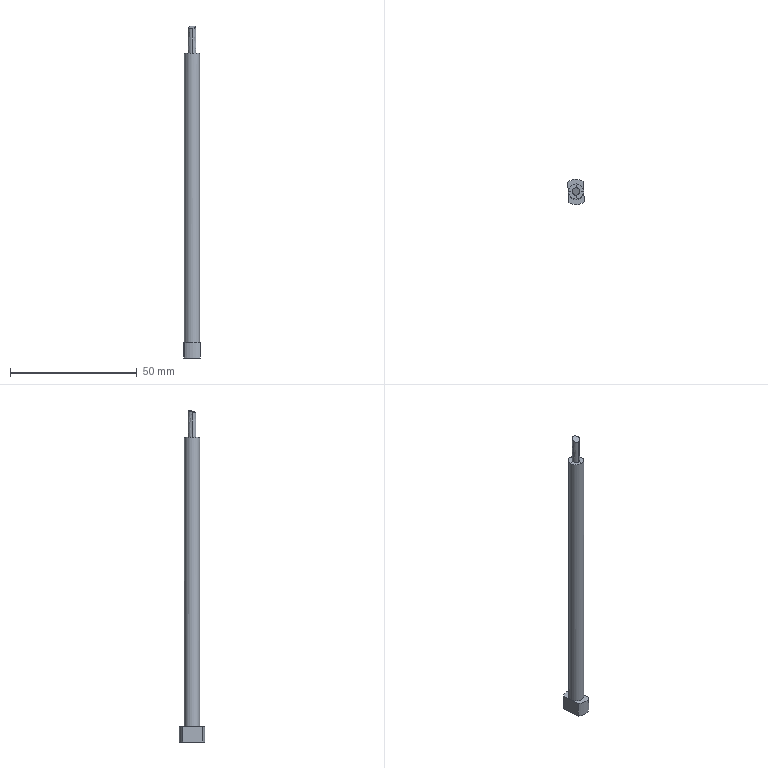Part | STEP file | 车灯-后视镜_id590_x_t | 1 solid | 16 faces | box 6.638 x 10 x 131.059 mm | volume 3645 mm3 | plane 8 | spline 5 | cylinder 3 | commonest cylinder face diameters 10 x2 6 x1
STEP:
#1=CARTESIAN_POINT('',(14.563,-72.692,45.992));
#2=VERTEX_POINT('',#1);
#3=CARTESIAN_POINT('',(11.568,-69.68,45.99));
#4=VERTEX_POINT('',#3);
#5=CARTESIAN_POINT('',(11.563,-72.687,45.992));
#6=DIRECTION('',(-0.00001772,-0.00006118,1.));
#7=DIRECTION('',(0.2782,0.9605,0.00006369));
#8=AXIS2_PLACEMENT_3D('',#5,#6,#7);
#9=ELLIPSE('',#8,3.,3.);
#10=EDGE_CURVE('',#2,#4,#9,.T.);
#11=ORIENTED_EDGE('',*,*,#10,.F.);
#12=CARTESIAN_POINT('',(11.575,-75.7,45.991));
#13=VERTEX_POINT('',#12);
#14=CARTESIAN_POINT('',(11.563,-72.687,45.992));
#15=DIRECTION('',(-0.00004877,0.00005142,-1.));
#16=DIRECTION('',(-0.6881,0.7256,0.00007087));
#17=AXIS2_PLACEMENT_3D('',#14,#15,#16);
#18=ELLIPSE('',#17,3.,3.);
#19=EDGE_CURVE('',#2,#13,#18,.T.);
#20=ORIENTED_EDGE('',*,*,#19,.T.);
#21=CARTESIAN_POINT('',(8.555,-72.692,45.989));
#22=VERTEX_POINT('',#21);
#23=CARTESIAN_POINT('',(8.555,-72.692,45.992));
#24=CARTESIAN_POINT('',(8.556,-73.526,45.992));
#25=CARTESIAN_POINT('',(8.85,-74.236,45.992));
#26=CARTESIAN_POINT('',(10.027,-75.412,45.992));
#27=CARTESIAN_POINT('',(10.738,-75.707,45.992));
#28=CARTESIAN_POINT('',(11.57,-75.707,45.992));
#29=B_SPLINE_CURVE_WITH_KNOTS('',3,(#23,#24,#25,#26,#27,#28),.UNSPECIFIED.,.F.,.F.,(4,2,4),(0.,0.5,1.),.UNSPECIFIED.);
#30=EDGE_CURVE('',#22,#13,#29,.T.);
#31=ORIENTED_EDGE('',*,*,#30,.F.);
#32=CARTESIAN_POINT('',(8.563,-72.692,45.992));
#33=CARTESIAN_POINT('',(8.562,-71.905,45.992));
#34=CARTESIAN_POINT('',(8.885,-71.122,45.992));
#35=CARTESIAN_POINT('',(9.998,-70.01,45.992));
#36=CARTESIAN_POINT('',(10.781,-69.686,45.992));
#37=CARTESIAN_POINT('',(11.568,-69.687,45.992));
#38=B_SPLINE_CURVE_WITH_KNOTS('',3,(#32,#33,#34,#35,#36,#37),.UNSPECIFIED.,.F.,.F.,(4,2,4),(0.,0.5,1.),.UNSPECIFIED.);
#39=EDGE_CURVE('',#22,#4,#38,.T.);
#40=ORIENTED_EDGE('',*,*,#39,.T.);
#41=EDGE_LOOP('',(#11,#20,#31,#40));
#42=FACE_BOUND('',#41,.T.);
#43=CARTESIAN_POINT('',(14.563,-72.687,-68.25));
#44=VERTEX_POINT('',#43);
#45=CARTESIAN_POINT('',(11.563,-72.687,-68.25));
#46=DIRECTION('',(0.,0.,-1.));
#47=DIRECTION('',(1.,0.,0.));
#48=AXIS2_PLACEMENT_3D('',#45,#46,#47);
#49=CIRCLE('',#48,3.);
#50=EDGE_CURVE('',#44,#44,#49,.T.);
#51=ORIENTED_EDGE('',*,*,#50,.F.);
#52=EDGE_LOOP('',(#51));
#53=FACE_BOUND('',#52,.T.);
#54=CARTESIAN_POINT('',(11.563,-72.687,45.992));
#55=DIRECTION('',(0.,0.,1.));
#56=DIRECTION('',(1.,0.,0.));
#57=AXIS2_PLACEMENT_3D('',#54,#55,#56);
#58=CYLINDRICAL_SURFACE('',#57,3.);
#59=ADVANCED_FACE('',(#42,#53),#58,.T.);
#60=CARTESIAN_POINT('',(11.567,-71.184,56.788));
#61=VERTEX_POINT('',#60);
#62=CARTESIAN_POINT('',(11.275,-71.215,56.744));
#63=VERTEX_POINT('',#62);
#64=CARTESIAN_POINT('',(11.567,-71.184,56.788));
#65=CARTESIAN_POINT('',(11.469,-71.195,56.774));
#66=CARTESIAN_POINT('',(11.372,-71.205,56.761));
#67=CARTESIAN_POINT('',(11.275,-71.216,56.747));
#68=B_SPLINE_CURVE_WITH_KNOTS('',3,(#64,#65,#66,#67),.UNSPECIFIED.,.F.,.F.,(4,4),(0.,1.),.UNSPECIFIED.);
#69=EDGE_CURVE('',#61,#63,#68,.T.);
#70=ORIENTED_EDGE('',*,*,#69,.T.);
#71=CARTESIAN_POINT('',(10.857,-71.372,56.641));
#72=VERTEX_POINT('',#71);
#73=CARTESIAN_POINT('',(11.275,-71.216,56.747));
#74=CARTESIAN_POINT('',(11.135,-71.269,56.714));
#75=CARTESIAN_POINT('',(10.995,-71.322,56.681));
#76=CARTESIAN_POINT('',(10.856,-71.374,56.648));
#77=B_SPLINE_CURVE_WITH_KNOTS('',3,(#73,#74,#75,#76),.UNSPECIFIED.,.F.,.F.,(4,4),(0.,1.),.UNSPECIFIED.);
#78=EDGE_CURVE('',#63,#72,#77,.T.);
#79=ORIENTED_EDGE('',*,*,#78,.T.);
#80=CARTESIAN_POINT('',(10.059,-72.692,56.102));
#81=VERTEX_POINT('',#80);
#82=CARTESIAN_POINT('',(10.856,-71.374,56.648));
#83=CARTESIAN_POINT('',(10.323,-71.672,56.488));
#84=CARTESIAN_POINT('',(10.059,-72.113,56.305));
#85=CARTESIAN_POINT('',(10.059,-72.692,56.102));
#86=B_SPLINE_CURVE_WITH_KNOTS('',3,(#82,#83,#84,#85),.UNSPECIFIED.,.F.,.F.,(4,4),(0.,1.),.UNSPECIFIED.);
#87=EDGE_CURVE('',#72,#81,#86,.T.);
#88=ORIENTED_EDGE('',*,*,#87,.T.);
#89=CARTESIAN_POINT('',(10.061,-72.772,56.074));
#90=VERTEX_POINT('',#89);
#91=CARTESIAN_POINT('',(10.059,-72.692,56.102));
#92=CARTESIAN_POINT('',(10.06,-72.719,56.093));
#93=CARTESIAN_POINT('',(10.061,-72.746,56.084));
#94=CARTESIAN_POINT('',(10.061,-72.772,56.074));
#95=B_SPLINE_CURVE_WITH_KNOTS('',3,(#91,#92,#93,#94),.UNSPECIFIED.,.F.,.F.,(4,4),(0.,1.),.UNSPECIFIED.);
#96=EDGE_CURVE('',#81,#90,#95,.T.);
#97=ORIENTED_EDGE('',*,*,#96,.T.);
#98=CARTESIAN_POINT('',(11.099,-74.121,55.708));
#99=VERTEX_POINT('',#98);
#100=CARTESIAN_POINT('',(10.061,-72.772,56.074));
#101=CARTESIAN_POINT('',(10.081,-73.101,55.961));
#102=CARTESIAN_POINT('',(10.2,-73.394,55.871));
#103=CARTESIAN_POINT('',(10.637,-73.911,55.735));
#104=CARTESIAN_POINT('',(10.831,-74.029,55.713));
#105=CARTESIAN_POINT('',(11.099,-74.121,55.708));
#106=B_SPLINE_CURVE_WITH_KNOTS('',3,(#100,#101,#102,#103,#104,#105),.UNSPECIFIED.,.F.,.F.,(4,2,4),(0.,0.5,1.),.UNSPECIFIED.);
#107=EDGE_CURVE('',#90,#99,#106,.T.);
#108=ORIENTED_EDGE('',*,*,#107,.T.);
#109=CARTESIAN_POINT('',(11.567,-74.199,55.727));
#110=VERTEX_POINT('',#109);
#111=CARTESIAN_POINT('',(11.099,-74.121,55.708));
#112=CARTESIAN_POINT('',(11.248,-74.172,55.705));
#113=CARTESIAN_POINT('',(11.404,-74.198,55.711));
#114=CARTESIAN_POINT('',(11.567,-74.199,55.727));
#115=B_SPLINE_CURVE_WITH_KNOTS('',3,(#111,#112,#113,#114),.UNSPECIFIED.,.F.,.F.,(4,4),(0.,1.),.UNSPECIFIED.);
#116=EDGE_CURVE('',#99,#110,#115,.T.);
#117=ORIENTED_EDGE('',*,*,#116,.T.);
#118=CARTESIAN_POINT('',(11.874,-74.165,55.772));
#119=VERTEX_POINT('',#118);
#120=CARTESIAN_POINT('',(11.567,-74.199,55.727));
#121=CARTESIAN_POINT('',(11.672,-74.199,55.738));
#122=CARTESIAN_POINT('',(11.774,-74.187,55.752));
#123=CARTESIAN_POINT('',(11.874,-74.165,55.77));
#124=B_SPLINE_CURVE_WITH_KNOTS('',3,(#120,#121,#122,#123),.UNSPECIFIED.,.F.,.F.,(4,4),(0.,1.),.UNSPECIFIED.);
#125=EDGE_CURVE('',#110,#119,#124,.T.);
#126=ORIENTED_EDGE('',*,*,#125,.T.);
#127=CARTESIAN_POINT('',(12.283,-74.008,55.873));
#128=VERTEX_POINT('',#127);
#129=CARTESIAN_POINT('',(11.874,-74.165,55.77));
#130=CARTESIAN_POINT('',(12.01,-74.111,55.802));
#131=CARTESIAN_POINT('',(12.147,-74.058,55.834));
#132=CARTESIAN_POINT('',(12.284,-74.005,55.866));
#133=B_SPLINE_CURVE_WITH_KNOTS('',3,(#129,#130,#131,#132),.UNSPECIFIED.,.F.,.F.,(4,4),(0.,1.),.UNSPECIFIED.);
#134=EDGE_CURVE('',#119,#128,#133,.T.);
#135=ORIENTED_EDGE('',*,*,#134,.T.);
#136=CARTESIAN_POINT('',(12.422,-73.921,55.918));
#137=VERTEX_POINT('',#136);
#138=CARTESIAN_POINT('',(12.284,-74.005,55.866));
#139=CARTESIAN_POINT('',(12.33,-73.976,55.881));
#140=CARTESIAN_POINT('',(12.376,-73.947,55.896));
#141=CARTESIAN_POINT('',(12.422,-73.918,55.911));
#142=B_SPLINE_CURVE_WITH_KNOTS('',3,(#138,#139,#140,#141),.UNSPECIFIED.,.F.,.F.,(4,4),(0.,1.),.UNSPECIFIED.);
#143=EDGE_CURVE('',#128,#137,#142,.T.);
#144=ORIENTED_EDGE('',*,*,#143,.T.);
#145=CARTESIAN_POINT('',(13.074,-72.692,56.408));
#146=VERTEX_POINT('',#145);
#147=CARTESIAN_POINT('',(12.422,-73.918,55.911));
#148=CARTESIAN_POINT('',(12.855,-73.609,56.063));
#149=CARTESIAN_POINT('',(13.074,-73.201,56.228));
#150=CARTESIAN_POINT('',(13.074,-72.692,56.408));
#151=B_SPLINE_CURVE_WITH_KNOTS('',3,(#147,#148,#149,#150),.UNSPECIFIED.,.F.,.F.,(4,4),(0.,1.),.UNSPECIFIED.);
#152=EDGE_CURVE('',#137,#146,#151,.T.);
#153=ORIENTED_EDGE('',*,*,#152,.T.);
#154=CARTESIAN_POINT('',(12.038,-71.263,56.808));
#155=VERTEX_POINT('',#154);
#156=CARTESIAN_POINT('',(13.074,-72.692,56.408));
#157=CARTESIAN_POINT('',(13.073,-72.055,56.633));
#158=CARTESIAN_POINT('',(12.654,-71.473,56.797));
#159=CARTESIAN_POINT('',(12.038,-71.263,56.809));
#160=B_SPLINE_CURVE_WITH_KNOTS('',3,(#156,#157,#158,#159),.UNSPECIFIED.,.F.,.F.,(4,4),(0.,1.),.UNSPECIFIED.);
#161=EDGE_CURVE('',#146,#155,#160,.T.);
#162=ORIENTED_EDGE('',*,*,#161,.T.);
#163=CARTESIAN_POINT('',(12.038,-71.263,56.809));
#164=CARTESIAN_POINT('',(11.887,-71.211,56.811));
#165=CARTESIAN_POINT('',(11.73,-71.185,56.804));
#166=CARTESIAN_POINT('',(11.567,-71.184,56.788));
#167=B_SPLINE_CURVE_WITH_KNOTS('',3,(#163,#164,#165,#166),.UNSPECIFIED.,.F.,.F.,(4,4),(0.,1.),.UNSPECIFIED.);
#168=EDGE_CURVE('',#155,#61,#167,.T.);
#169=ORIENTED_EDGE('',*,*,#168,.T.);
#170=EDGE_LOOP('',(#70,#79,#88,#97,#108,#117,#126,#135,#144,#153,#162,#169));
#171=FACE_OUTER_BOUND('',#170,.T.);
#172=CARTESIAN_POINT('',(13.104,-71.095,56.968));
#173=CARTESIAN_POINT('',(12.07,-71.139,56.858));
#174=CARTESIAN_POINT('',(11.046,-71.186,56.737));
#175=CARTESIAN_POINT('',(10.034,-71.237,56.604));
#176=CARTESIAN_POINT('',(13.098,-72.12,56.614));
#177=CARTESIAN_POINT('',(12.067,-72.165,56.505));
#178=CARTESIAN_POINT('',(11.047,-72.213,56.384));
#179=CARTESIAN_POINT('',(10.039,-72.264,56.252));
#180=CARTESIAN_POINT('',(13.091,-73.139,56.254));
#181=CARTESIAN_POINT('',(12.064,-73.184,56.145));
#182=CARTESIAN_POINT('',(11.048,-73.233,56.026));
#183=CARTESIAN_POINT('',(10.043,-73.284,55.895));
#184=CARTESIAN_POINT('',(13.083,-74.15,55.887));
#185=CARTESIAN_POINT('',(12.06,-74.196,55.78));
#186=CARTESIAN_POINT('',(11.048,-74.245,55.662));
#187=CARTESIAN_POINT('',(10.048,-74.297,55.532));
#188=B_SPLINE_SURFACE_WITH_KNOTS('',3,3,((#172,#173,#174,#175),(#176,#177,#178,#179),(#180,#181,#182,#183),(#184,#185,#186,#187)),.UNSPECIFIED.,.F.,.F.,.F.,(4,4),(4,4),(0.,1.),(0.,1.),.UNSPECIFIED.);
#189=ADVANCED_FACE('',(#171),#188,.F.);
#190=CARTESIAN_POINT('',(10.06,-72.692,45.992));
#191=VERTEX_POINT('',#190);
#192=CARTESIAN_POINT('',(10.06,-72.692,45.992));
#193=CARTESIAN_POINT('',(10.059,-72.692,56.102));
#194=B_SPLINE_CURVE_WITH_KNOTS('',1,(#192,#193),.UNSPECIFIED.,.F.,.F.,(2,2),(0.,1.),.UNSPECIFIED.);
#195=EDGE_CURVE('',#191,#81,#194,.T.);
#196=ORIENTED_EDGE('',*,*,#195,.T.);
#197=ORIENTED_EDGE('',*,*,#87,.F.);
#198=ORIENTED_EDGE('',*,*,#78,.F.);
#199=ORIENTED_EDGE('',*,*,#69,.F.);
#200=CARTESIAN_POINT('',(11.568,-71.184,45.992));
#201=VERTEX_POINT('',#200);
#202=CARTESIAN_POINT('',(11.567,-71.184,56.788));
#203=CARTESIAN_POINT('',(11.568,-71.184,45.992));
#204=B_SPLINE_CURVE_WITH_KNOTS('',1,(#202,#203),.UNSPECIFIED.,.F.,.F.,(2,2),(0.,1.),.UNSPECIFIED.);
#205=EDGE_CURVE('',#61,#201,#204,.T.);
#206=ORIENTED_EDGE('',*,*,#205,.T.);
#207=CARTESIAN_POINT('',(11.568,-71.184,45.992));
#208=CARTESIAN_POINT('',(10.753,-71.184,45.992));
#209=CARTESIAN_POINT('',(10.06,-71.88,45.992));
#210=CARTESIAN_POINT('',(10.06,-72.692,45.992));
#211=B_SPLINE_CURVE_WITH_KNOTS('',3,(#207,#208,#209,#210),.UNSPECIFIED.,.F.,.F.,(4,4),(0.,1.),.UNSPECIFIED.);
#212=EDGE_CURVE('',#201,#191,#211,.T.);
#213=ORIENTED_EDGE('',*,*,#212,.T.);
#214=EDGE_LOOP('',(#196,#197,#198,#199,#206,#213));
#215=FACE_OUTER_BOUND('',#214,.T.);
#216=CARTESIAN_POINT('',(11.568,-71.184,45.992));
#217=CARTESIAN_POINT('',(11.567,-71.184,56.853));
#218=CARTESIAN_POINT('',(10.753,-71.184,45.992));
#219=CARTESIAN_POINT('',(10.751,-71.184,56.853));
#220=CARTESIAN_POINT('',(10.06,-71.88,45.992));
#221=CARTESIAN_POINT('',(10.059,-71.88,56.853));
#222=CARTESIAN_POINT('',(10.06,-72.692,45.992));
#223=CARTESIAN_POINT('',(10.059,-72.692,56.853));
#224=B_SPLINE_SURFACE_WITH_KNOTS('',3,1,((#216,#217),(#218,#219),(#220,#221),(#222,#223)),.UNSPECIFIED.,.F.,.F.,.F.,(4,4),(2,2),(0.,1.),(0.,1.),.UNSPECIFIED.);
#225=ADVANCED_FACE('',(#215),#224,.T.);
#226=CARTESIAN_POINT('',(13.075,-72.692,45.992));
#227=VERTEX_POINT('',#226);
#228=CARTESIAN_POINT('',(13.074,-72.692,56.408));
#229=CARTESIAN_POINT('',(13.074,-72.692,52.936));
#230=CARTESIAN_POINT('',(13.075,-72.692,49.464));
#231=CARTESIAN_POINT('',(13.075,-72.692,45.992));
#232=B_SPLINE_CURVE_WITH_KNOTS('',3,(#228,#229,#230,#231),.UNSPECIFIED.,.F.,.F.,(4,4),(0.,1.),.UNSPECIFIED.);
#233=EDGE_CURVE('',#146,#227,#232,.T.);
#234=ORIENTED_EDGE('',*,*,#233,.F.);
#235=ORIENTED_EDGE('',*,*,#152,.F.);
#236=ORIENTED_EDGE('',*,*,#143,.F.);
#237=ORIENTED_EDGE('',*,*,#134,.F.);
#238=ORIENTED_EDGE('',*,*,#125,.F.);
#239=CARTESIAN_POINT('',(11.568,-74.199,45.992));
#240=VERTEX_POINT('',#239);
#241=CARTESIAN_POINT('',(11.568,-74.199,45.992));
#242=CARTESIAN_POINT('',(11.567,-74.199,55.727));
#243=B_SPLINE_CURVE_WITH_KNOTS('',1,(#241,#242),.UNSPECIFIED.,.F.,.F.,(2,2),(0.,1.),.UNSPECIFIED.);
#244=EDGE_CURVE('',#240,#110,#243,.T.);
#245=ORIENTED_EDGE('',*,*,#244,.F.);
#246=CARTESIAN_POINT('',(11.568,-74.199,45.992));
#247=CARTESIAN_POINT('',(12.383,-74.199,45.992));
#248=CARTESIAN_POINT('',(13.075,-73.504,45.992));
#249=CARTESIAN_POINT('',(13.075,-72.692,45.992));
#250=B_SPLINE_CURVE_WITH_KNOTS('',3,(#246,#247,#248,#249),.UNSPECIFIED.,.F.,.F.,(4,4),(0.,1.),.UNSPECIFIED.);
#251=EDGE_CURVE('',#240,#227,#250,.T.);
#252=ORIENTED_EDGE('',*,*,#251,.T.);
#253=EDGE_LOOP('',(#234,#235,#236,#237,#238,#245,#252));
#254=FACE_OUTER_BOUND('',#253,.T.);
#255=CARTESIAN_POINT('',(11.568,-74.199,45.992));
#256=CARTESIAN_POINT('',(11.567,-74.199,56.47));
#257=CARTESIAN_POINT('',(12.383,-74.199,45.992));
#258=CARTESIAN_POINT('',(12.382,-74.199,56.47));
#259=CARTESIAN_POINT('',(13.075,-73.504,45.992));
#260=CARTESIAN_POINT('',(13.074,-73.504,56.47));
#261=CARTESIAN_POINT('',(13.075,-72.692,45.992));
#262=CARTESIAN_POINT('',(13.074,-72.692,56.47));
#263=B_SPLINE_SURFACE_WITH_KNOTS('',3,1,((#255,#256),(#257,#258),(#259,#260),(#261,#262)),.UNSPECIFIED.,.F.,.F.,.F.,(4,4),(2,2),(0.,1.),(0.,1.),.UNSPECIFIED.);
#264=ADVANCED_FACE('',(#254),#263,.T.);
#265=CARTESIAN_POINT('',(11.568,-71.184,45.992));
#266=CARTESIAN_POINT('',(12.38,-71.185,45.992));
#267=CARTESIAN_POINT('',(13.075,-71.887,45.992));
#268=CARTESIAN_POINT('',(13.075,-72.692,45.992));
#269=B_SPLINE_CURVE_WITH_KNOTS('',3,(#265,#266,#267,#268),.UNSPECIFIED.,.F.,.F.,(4,4),(0.,1.),.UNSPECIFIED.);
#270=EDGE_CURVE('',#201,#227,#269,.T.);
#271=ORIENTED_EDGE('',*,*,#270,.F.);
#272=ORIENTED_EDGE('',*,*,#205,.F.);
#273=ORIENTED_EDGE('',*,*,#168,.F.);
#274=ORIENTED_EDGE('',*,*,#161,.F.);
#275=ORIENTED_EDGE('',*,*,#233,.T.);
#276=EDGE_LOOP('',(#271,#272,#273,#274,#275));
#277=FACE_OUTER_BOUND('',#276,.T.);
#278=CARTESIAN_POINT('',(11.568,-71.184,45.992));
#279=CARTESIAN_POINT('',(11.567,-71.184,49.62));
#280=CARTESIAN_POINT('',(11.567,-71.184,53.249));
#281=CARTESIAN_POINT('',(11.567,-71.184,56.878));
#282=CARTESIAN_POINT('',(12.388,-71.184,45.992));
#283=CARTESIAN_POINT('',(12.388,-71.184,49.62));
#284=CARTESIAN_POINT('',(12.388,-71.184,53.249));
#285=CARTESIAN_POINT('',(12.387,-71.184,56.878));
#286=CARTESIAN_POINT('',(13.075,-71.871,45.992));
#287=CARTESIAN_POINT('',(13.075,-71.871,49.62));
#288=CARTESIAN_POINT('',(13.074,-71.871,53.249));
#289=CARTESIAN_POINT('',(13.074,-71.871,56.878));
#290=CARTESIAN_POINT('',(13.075,-72.692,45.992));
#291=CARTESIAN_POINT('',(13.075,-72.692,49.62));
#292=CARTESIAN_POINT('',(13.074,-72.692,53.249));
#293=CARTESIAN_POINT('',(13.074,-72.692,56.878));
#294=B_SPLINE_SURFACE_WITH_KNOTS('',3,3,((#278,#279,#280,#281),(#282,#283,#284,#285),(#286,#287,#288,#289),(#290,#291,#292,#293)),.UNSPECIFIED.,.F.,.F.,.F.,(4,4),(4,4),(0.,1.),(0.,1.),.UNSPECIFIED.);
#295=ADVANCED_FACE('',(#277),#294,.F.);
#296=ORIENTED_EDGE('',*,*,#244,.T.);
#297=ORIENTED_EDGE('',*,*,#116,.F.);
#298=ORIENTED_EDGE('',*,*,#107,.F.);
#299=ORIENTED_EDGE('',*,*,#96,.F.);
#300=ORIENTED_EDGE('',*,*,#195,.F.);
#301=CARTESIAN_POINT('',(10.06,-72.692,45.992));
#302=CARTESIAN_POINT('',(10.06,-73.507,45.992));
#303=CARTESIAN_POINT('',(10.756,-74.199,45.992));
#304=CARTESIAN_POINT('',(11.568,-74.199,45.992));
#305=B_SPLINE_CURVE_WITH_KNOTS('',3,(#301,#302,#303,#304),.UNSPECIFIED.,.F.,.F.,(4,4),(0.,1.),.UNSPECIFIED.);
#306=EDGE_CURVE('',#191,#240,#305,.T.);
#307=ORIENTED_EDGE('',*,*,#306,.T.);
#308=EDGE_LOOP('',(#296,#297,#298,#299,#300,#307));
#309=FACE_OUTER_BOUND('',#308,.T.);
#310=CARTESIAN_POINT('',(10.06,-72.692,45.992));
#311=CARTESIAN_POINT('',(10.059,-72.692,56.163));
#312=CARTESIAN_POINT('',(10.06,-73.507,45.992));
#313=CARTESIAN_POINT('',(10.059,-73.507,56.163));
#314=CARTESIAN_POINT('',(10.756,-74.199,45.992));
#315=CARTESIAN_POINT('',(10.755,-74.199,56.163));
#316=CARTESIAN_POINT('',(11.568,-74.199,45.992));
#317=CARTESIAN_POINT('',(11.567,-74.199,56.163));
#318=B_SPLINE_SURFACE_WITH_KNOTS('',3,1,((#310,#311),(#312,#313),(#314,#315),(#316,#317)),.UNSPECIFIED.,.F.,.F.,.F.,(4,4),(2,2),(0.,1.),(0.,1.),.UNSPECIFIED.);
#319=ADVANCED_FACE('',(#309),#318,.T.);
#320=ORIENTED_EDGE('',*,*,#306,.F.);
#321=CARTESIAN_POINT('',(8.543,-72.692,45.992));
#322=CARTESIAN_POINT('',(9.049,-72.692,45.992));
#323=CARTESIAN_POINT('',(9.555,-72.692,45.992));
#324=CARTESIAN_POINT('',(10.06,-72.692,45.992));
#325=B_SPLINE_CURVE_WITH_KNOTS('',3,(#321,#322,#323,#324),.UNSPECIFIED.,.F.,.F.,(4,4),(0.,1.),.UNSPECIFIED.);
#326=EDGE_CURVE('',#22,#191,#325,.T.);
#327=ORIENTED_EDGE('',*,*,#326,.F.);
#328=ORIENTED_EDGE('',*,*,#30,.T.);
#329=CARTESIAN_POINT('',(11.576,-75.719,45.992));
#330=CARTESIAN_POINT('',(11.573,-75.212,45.992));
#331=CARTESIAN_POINT('',(11.571,-74.706,45.992));
#332=CARTESIAN_POINT('',(11.568,-74.199,45.992));
#333=B_SPLINE_CURVE_WITH_KNOTS('',3,(#329,#330,#331,#332),.UNSPECIFIED.,.F.,.F.,(4,4),(0.,1.),.UNSPECIFIED.);
#334=EDGE_CURVE('',#13,#240,#333,.T.);
#335=ORIENTED_EDGE('',*,*,#334,.T.);
#336=EDGE_LOOP('',(#320,#327,#328,#335));
#337=FACE_OUTER_BOUND('',#336,.T.);
#338=CARTESIAN_POINT('',(10.06,-72.692,45.992));
#339=DIRECTION('',(0.,0.,1.));
#340=DIRECTION('',(0.7071,-0.7071,0.));
#341=AXIS2_PLACEMENT_3D('',#338,#339,#340);
#342=PLANE('',#341);
#343=ADVANCED_FACE('',(#337),#342,.T.);
#344=CARTESIAN_POINT('',(13.075,-72.692,45.992));
#345=CARTESIAN_POINT('',(13.571,-72.692,45.992));
#346=CARTESIAN_POINT('',(14.067,-72.692,45.992));
#347=CARTESIAN_POINT('',(14.563,-72.692,45.992));
#348=B_SPLINE_CURVE_WITH_KNOTS('',3,(#344,#345,#346,#347),.UNSPECIFIED.,.F.,.F.,(4,4),(0.,1.),.UNSPECIFIED.);
#349=EDGE_CURVE('',#227,#2,#348,.T.);
#350=ORIENTED_EDGE('',*,*,#349,.T.);
#351=ORIENTED_EDGE('',*,*,#10,.T.);
#352=CARTESIAN_POINT('',(11.568,-69.687,45.992));
#353=CARTESIAN_POINT('',(11.568,-70.186,45.992));
#354=CARTESIAN_POINT('',(11.568,-70.685,45.992));
#355=CARTESIAN_POINT('',(11.568,-71.184,45.992));
#356=B_SPLINE_CURVE_WITH_KNOTS('',3,(#352,#353,#354,#355),.UNSPECIFIED.,.F.,.F.,(4,4),(0.,1.),.UNSPECIFIED.);
#357=EDGE_CURVE('',#4,#201,#356,.T.);
#358=ORIENTED_EDGE('',*,*,#357,.T.);
#359=ORIENTED_EDGE('',*,*,#270,.T.);
#360=EDGE_LOOP('',(#350,#351,#358,#359));
#361=FACE_OUTER_BOUND('',#360,.T.);
#362=CARTESIAN_POINT('',(13.199,-71.063,45.992));
#363=DIRECTION('',(-0.00001772,-0.00006118,1.));
#364=DIRECTION('',(-0.000003024,-1.,-0.00006118));
#365=AXIS2_PLACEMENT_3D('',#362,#363,#364);
#366=PLANE('',#365);
#367=ADVANCED_FACE('',(#361),#366,.T.);
#368=ORIENTED_EDGE('',*,*,#19,.F.);
#369=ORIENTED_EDGE('',*,*,#349,.F.);
#370=ORIENTED_EDGE('',*,*,#251,.F.);
#371=ORIENTED_EDGE('',*,*,#334,.F.);
#372=EDGE_LOOP('',(#368,#369,#370,#371));
#373=FACE_OUTER_BOUND('',#372,.T.);
#374=CARTESIAN_POINT('',(13.202,-74.318,45.992));
#375=DIRECTION('',(-0.00004877,0.00005142,-1.));
#376=DIRECTION('',(0.000002542,1.,0.00005142));
#377=AXIS2_PLACEMENT_3D('',#374,#375,#376);
#378=PLANE('',#377);
#379=ADVANCED_FACE('',(#373),#378,.F.);
#380=ORIENTED_EDGE('',*,*,#39,.F.);
#381=ORIENTED_EDGE('',*,*,#326,.T.);
#382=ORIENTED_EDGE('',*,*,#212,.F.);
#383=ORIENTED_EDGE('',*,*,#357,.F.);
#384=EDGE_LOOP('',(#380,#381,#382,#383));
#385=FACE_OUTER_BOUND('',#384,.T.);
#386=CARTESIAN_POINT('',(9.937,-71.061,45.992));
#387=DIRECTION('',(-0.00002916,-0.00001772,-1.));
#388=DIRECTION('',(-0.000000876,1.,-0.00001772));
#389=AXIS2_PLACEMENT_3D('',#386,#387,#388);
#390=PLANE('',#389);
#391=ADVANCED_FACE('',(#385),#390,.F.);
#392=CARTESIAN_POINT('',(14.871,-76.437,-68.25));
#393=VERTEX_POINT('',#392);
#394=CARTESIAN_POINT('',(14.871,-76.437,-74.25));
#395=VERTEX_POINT('',#394);
#396=CARTESIAN_POINT('',(14.871,-76.437,-68.25));
#397=DIRECTION('',(0.,0.,-1.));
#398=VECTOR('',#397,1.);
#399=LINE('',#396,#398);
#400=EDGE_CURVE('',#393,#395,#399,.T.);
#401=ORIENTED_EDGE('',*,*,#400,.F.);
#402=CARTESIAN_POINT('',(8.784,-76.844,-68.25));
#403=VERTEX_POINT('',#402);
#404=CARTESIAN_POINT('',(11.563,-72.687,-68.25));
#405=DIRECTION('',(0.,0.,-1.));
#406=DIRECTION('',(-1.,0.,0.));
#407=AXIS2_PLACEMENT_3D('',#404,#405,#406);
#408=CIRCLE('',#407,5.);
#409=EDGE_CURVE('',#393,#403,#408,.T.);
#410=ORIENTED_EDGE('',*,*,#409,.T.);
#411=CARTESIAN_POINT('',(8.784,-76.844,-74.25));
#412=VERTEX_POINT('',#411);
#413=CARTESIAN_POINT('',(8.784,-76.844,-74.25));
#414=DIRECTION('',(0.,0.,1.));
#415=VECTOR('',#414,1.);
#416=LINE('',#413,#415);
#417=EDGE_CURVE('',#412,#403,#416,.T.);
#418=ORIENTED_EDGE('',*,*,#417,.F.);
#419=CARTESIAN_POINT('',(11.563,-72.687,-74.25));
#420=DIRECTION('',(0.,0.,1.));
#421=DIRECTION('',(1.,0.,0.));
#422=AXIS2_PLACEMENT_3D('',#419,#420,#421);
#423=CIRCLE('',#422,5.);
#424=EDGE_CURVE('',#412,#395,#423,.T.);
#425=ORIENTED_EDGE('',*,*,#424,.T.);
#426=EDGE_LOOP('',(#401,#410,#418,#425));
#427=FACE_OUTER_BOUND('',#426,.T.);
#428=CARTESIAN_POINT('',(11.563,-72.687,-74.25));
#429=DIRECTION('',(0.,0.,1.));
#430=DIRECTION('',(1.,0.,0.));
#431=AXIS2_PLACEMENT_3D('',#428,#429,#430);
#432=CYLINDRICAL_SURFACE('',#431,5.);
#433=ADVANCED_FACE('',(#427),#432,.T.);
#434=CARTESIAN_POINT('',(14.317,-68.514,-68.25));
#435=VERTEX_POINT('',#434);
#436=CARTESIAN_POINT('',(14.594,-72.475,-68.25));
#437=DIRECTION('',(0.06976,-0.9976,0.));
#438=VECTOR('',#437,1.);
#439=LINE('',#436,#438);
#440=EDGE_CURVE('',#435,#393,#439,.T.);
#441=ORIENTED_EDGE('',*,*,#440,.F.);
#442=CARTESIAN_POINT('',(8.233,-68.958,-68.25));
#443=VERTEX_POINT('',#442);
#444=CARTESIAN_POINT('',(11.563,-72.687,-68.25));
#445=DIRECTION('',(0.,0.,-1.));
#446=DIRECTION('',(-1.,0.,0.));
#447=AXIS2_PLACEMENT_3D('',#444,#445,#446);
#448=CIRCLE('',#447,5.);
#449=EDGE_CURVE('',#443,#435,#448,.T.);
#450=ORIENTED_EDGE('',*,*,#449,.F.);
#451=CARTESIAN_POINT('',(8.509,-72.901,-68.25));
#452=DIRECTION('',(-0.06976,0.9976,0.));
#453=VECTOR('',#452,1.);
#454=LINE('',#451,#453);
#455=EDGE_CURVE('',#403,#443,#454,.T.);
#456=ORIENTED_EDGE('',*,*,#455,.F.);
#457=ORIENTED_EDGE('',*,*,#409,.F.);
#458=EDGE_LOOP('',(#441,#450,#456,#457));
#459=FACE_BOUND('',#458,.T.);
#460=ORIENTED_EDGE('',*,*,#50,.T.);
#461=EDGE_LOOP('',(#460));
#462=FACE_BOUND('',#461,.T.);
#463=CARTESIAN_POINT('',(11.563,-72.687,-68.25));
#464=DIRECTION('',(0.,0.,1.));
#465=DIRECTION('',(1.,0.,0.));
#466=AXIS2_PLACEMENT_3D('',#463,#464,#465);
#467=PLANE('',#466);
#468=ADVANCED_FACE('',(#459,#462),#467,.T.);
#469=CARTESIAN_POINT('',(14.317,-68.514,-74.25));
#470=VERTEX_POINT('',#469);
#471=CARTESIAN_POINT('',(14.317,-68.514,-74.25));
#472=DIRECTION('',(0.,0.,1.));
#473=VECTOR('',#472,1.);
#474=LINE('',#471,#473);
#475=EDGE_CURVE('',#470,#435,#474,.T.);
#476=ORIENTED_EDGE('',*,*,#475,.F.);
#477=CARTESIAN_POINT('',(8.233,-68.958,-74.25));
#478=VERTEX_POINT('',#477);
#479=CARTESIAN_POINT('',(11.563,-72.687,-74.25));
#480=DIRECTION('',(0.,0.,1.));
#481=DIRECTION('',(1.,0.,0.));
#482=AXIS2_PLACEMENT_3D('',#479,#480,#481);
#483=CIRCLE('',#482,5.);
#484=EDGE_CURVE('',#470,#478,#483,.T.);
#485=ORIENTED_EDGE('',*,*,#484,.T.);
#486=CARTESIAN_POINT('',(8.233,-68.958,-68.25));
#487=DIRECTION('',(0.,0.,-1.));
#488=VECTOR('',#487,1.);
#489=LINE('',#486,#488);
#490=EDGE_CURVE('',#443,#478,#489,.T.);
#491=ORIENTED_EDGE('',*,*,#490,.F.);
#492=ORIENTED_EDGE('',*,*,#449,.T.);
#493=EDGE_LOOP('',(#476,#485,#491,#492));
#494=FACE_OUTER_BOUND('',#493,.T.);
#495=CARTESIAN_POINT('',(11.563,-72.687,-74.25));
#496=DIRECTION('',(0.,0.,1.));
#497=DIRECTION('',(1.,0.,0.));
#498=AXIS2_PLACEMENT_3D('',#495,#496,#497);
#499=CYLINDRICAL_SURFACE('',#498,5.);
#500=ADVANCED_FACE('',(#494),#499,.T.);
#501=CARTESIAN_POINT('',(9.553,-0.3809,-74.25));
#502=DIRECTION('',(-0.06976,0.9976,0.));
#503=VECTOR('',#502,1.);
#504=LINE('',#501,#503);
#505=EDGE_CURVE('',#395,#470,#504,.T.);
#506=ORIENTED_EDGE('',*,*,#505,.F.);
#507=ORIENTED_EDGE('',*,*,#424,.F.);
#508=CARTESIAN_POINT('',(3.467,-0.8064,-74.25));
#509=DIRECTION('',(0.06976,-0.9976,0.));
#510=VECTOR('',#509,1.);
#511=LINE('',#508,#510);
#512=EDGE_CURVE('',#478,#412,#511,.T.);
#513=ORIENTED_EDGE('',*,*,#512,.F.);
#514=ORIENTED_EDGE('',*,*,#484,.F.);
#515=EDGE_LOOP('',(#506,#507,#513,#514));
#516=FACE_OUTER_BOUND('',#515,.T.);
#517=CARTESIAN_POINT('',(15.,0.,-74.25));
#518=DIRECTION('',(0.,0.,-1.));
#519=DIRECTION('',(-1.,0.,0.));
#520=AXIS2_PLACEMENT_3D('',#517,#518,#519);
#521=PLANE('',#520);
#522=ADVANCED_FACE('',(#516),#521,.T.);
#523=ORIENTED_EDGE('',*,*,#455,.T.);
#524=ORIENTED_EDGE('',*,*,#490,.T.);
#525=ORIENTED_EDGE('',*,*,#512,.T.);
#526=ORIENTED_EDGE('',*,*,#417,.T.);
#527=EDGE_LOOP('',(#523,#524,#525,#526));
#528=FACE_OUTER_BOUND('',#527,.T.);
#529=CARTESIAN_POINT('',(8.521,-73.081,-74.25));
#530=DIRECTION('',(0.9976,0.06976,0.));
#531=DIRECTION('',(-0.06976,0.9976,0.));
#532=AXIS2_PLACEMENT_3D('',#529,#530,#531);
#533=PLANE('',#532);
#534=ADVANCED_FACE('',(#528),#533,.F.);
#535=ORIENTED_EDGE('',*,*,#440,.T.);
#536=ORIENTED_EDGE('',*,*,#400,.T.);
#537=ORIENTED_EDGE('',*,*,#505,.T.);
#538=ORIENTED_EDGE('',*,*,#475,.T.);
#539=EDGE_LOOP('',(#535,#536,#537,#538));
#540=FACE_OUTER_BOUND('',#539,.T.);
#541=CARTESIAN_POINT('',(14.594,-72.475,-71.25));
#542=DIRECTION('',(-0.9976,-0.06976,0.));
#543=DIRECTION('',(0.06976,-0.9976,0.));
#544=AXIS2_PLACEMENT_3D('',#541,#542,#543);
#545=PLANE('',#544);
#546=ADVANCED_FACE('',(#540),#545,.F.);
#547=CLOSED_SHELL('',(#59,#189,#225,#264,#295,#319,#343,#367,#379,#391,#433,#468,#500,#522,#534,#546));
#548=MANIFOLD_SOLID_BREP('',#547);
#549=(LENGTH_UNIT()NAMED_UNIT(*)SI_UNIT(.MILLI.,.METRE.));
#550=UNCERTAINTY_MEASURE_WITH_UNIT(LENGTH_MEASURE(0.07465),#549,'','');
#551=(NAMED_UNIT(*)PLANE_ANGLE_UNIT()SI_UNIT($,.RADIAN.));
#552=PLANE_ANGLE_MEASURE_WITH_UNIT(PLANE_ANGLE_MEASURE(0.01745),#551);
#553=DIMENSIONAL_EXPONENTS(0.,0.,0.,0.,0.,0.,0.);
#554=(CONVERSION_BASED_UNIT('DEGREE',#552)NAMED_UNIT(#553)PLANE_ANGLE_UNIT());
#555=(NAMED_UNIT(*)SI_UNIT($,.STERADIAN.)SOLID_ANGLE_UNIT());
#556=(GEOMETRIC_REPRESENTATION_CONTEXT(3)GLOBAL_UNCERTAINTY_ASSIGNED_CONTEXT((#550))GLOBAL_UNIT_ASSIGNED_CONTEXT((#549,#554,#555))REPRESENTATION_CONTEXT('',''));
#557=ADVANCED_BREP_SHAPE_REPRESENTATION('',(#548),#556);